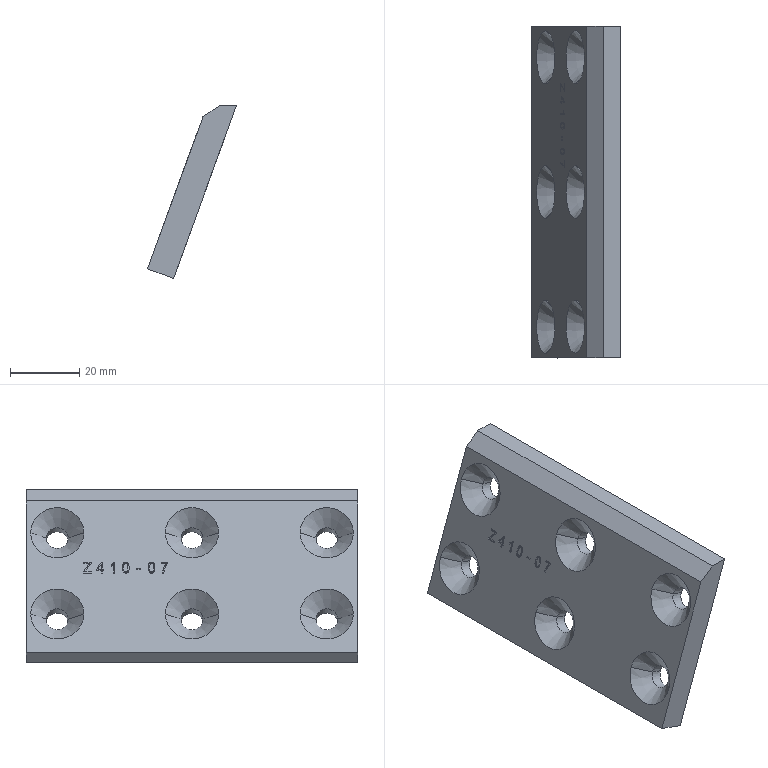Part | Creo | 1 solid | 131 faces | box 25.716 x 96 x 50 mm | volume 35834 mm3 | other 53 | plane 51 | cylinder 15 | cone 12 | commonest cylinder face diameters 6.4 x12 11.472 x1 11.957 x1 45.582 x1